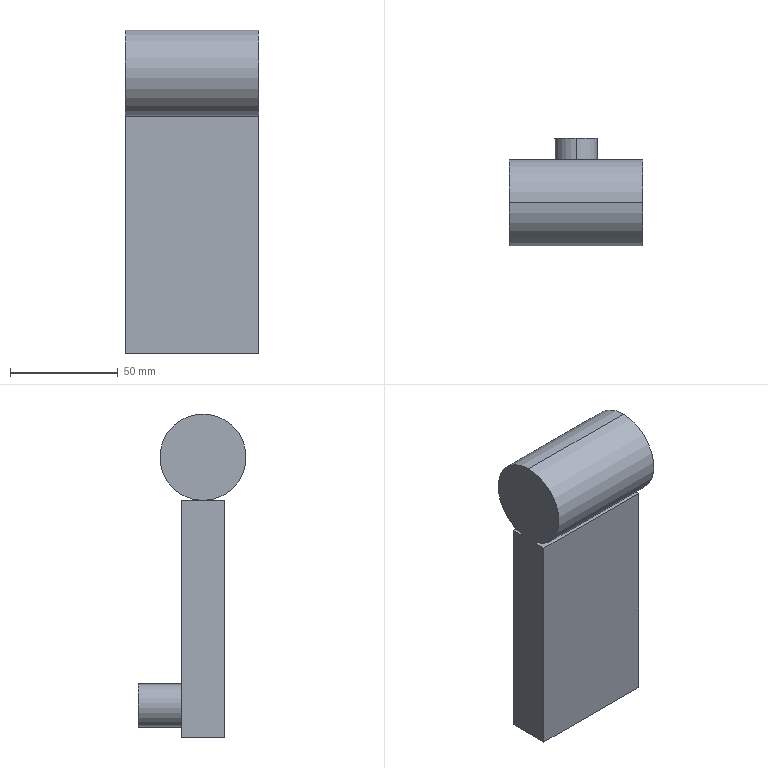Part | SolidWorks | features ICE 2, Extrusion 1 | 2 solids | 13 faces | box 62 x 50 x 150 mm | volume 220595 mm3 | plane 9 | cylinder 4 | commonest cylinder face diameters 20 x2 40 x2
STEP:
#1=CARTESIAN_POINT('',(-31.,0.,150.));
#2=VERTEX_POINT('',#1);
#3=CARTESIAN_POINT('',(-31.,0.,110.));
#4=VERTEX_POINT('',#3);
#5=CARTESIAN_POINT('',(-31.,0.,130.));
#6=DIRECTION('',(-1.,0.,0.));
#7=DIRECTION('',(0.,0.,-1.));
#8=AXIS2_PLACEMENT_3D('',#5,#6,#7);
#9=CIRCLE('',#8,20.);
#10=EDGE_CURVE('',#2,#4,#9,.T.);
#11=ORIENTED_EDGE('',*,*,#10,.F.);
#12=CARTESIAN_POINT('',(31.,0.,150.));
#13=VERTEX_POINT('',#12);
#14=CARTESIAN_POINT('',(-87.569,0.,150.));
#15=DIRECTION('',(1.,0.,0.));
#16=VECTOR('',#15,1000.);
#17=LINE('',#14,#16);
#18=EDGE_CURVE('',#2,#13,#17,.T.);
#19=ORIENTED_EDGE('',*,*,#18,.T.);
#20=CARTESIAN_POINT('',(31.,0.,110.));
#21=VERTEX_POINT('',#20);
#22=CARTESIAN_POINT('',(31.,0.,130.));
#23=DIRECTION('',(1.,0.,0.));
#24=DIRECTION('',(0.,0.,-1.));
#25=AXIS2_PLACEMENT_3D('',#22,#23,#24);
#26=CIRCLE('',#25,20.);
#27=EDGE_CURVE('',#21,#13,#26,.T.);
#28=ORIENTED_EDGE('',*,*,#27,.F.);
#29=CARTESIAN_POINT('',(-87.569,0.,110.));
#30=DIRECTION('',(1.,0.,0.));
#31=VECTOR('',#30,1000.);
#32=LINE('',#29,#31);
#33=EDGE_CURVE('',#4,#21,#32,.T.);
#34=ORIENTED_EDGE('',*,*,#33,.F.);
#35=EDGE_LOOP('',(#11,#19,#28,#34));
#36=FACE_OUTER_BOUND('',#35,.T.);
#37=CARTESIAN_POINT('',(-87.569,0.,130.));
#38=DIRECTION('',(1.,0.,0.));
#39=DIRECTION('',(0.,0.,-1.));
#40=AXIS2_PLACEMENT_3D('',#37,#38,#39);
#41=CYLINDRICAL_SURFACE('',#40,20.);
#42=ADVANCED_FACE('',(#36),#41,.T.);
#43=ORIENTED_EDGE('',*,*,#18,.F.);
#44=CARTESIAN_POINT('',(-31.,0.,130.));
#45=DIRECTION('',(-1.,0.,0.));
#46=DIRECTION('',(0.,0.,-1.));
#47=AXIS2_PLACEMENT_3D('',#44,#45,#46);
#48=CIRCLE('',#47,20.);
#49=EDGE_CURVE('',#4,#2,#48,.T.);
#50=ORIENTED_EDGE('',*,*,#49,.F.);
#51=ORIENTED_EDGE('',*,*,#33,.T.);
#52=CARTESIAN_POINT('',(31.,0.,130.));
#53=DIRECTION('',(1.,0.,0.));
#54=DIRECTION('',(0.,0.,-1.));
#55=AXIS2_PLACEMENT_3D('',#52,#53,#54);
#56=CIRCLE('',#55,20.);
#57=EDGE_CURVE('',#13,#21,#56,.T.);
#58=ORIENTED_EDGE('',*,*,#57,.F.);
#59=EDGE_LOOP('',(#43,#50,#51,#58));
#60=FACE_OUTER_BOUND('',#59,.T.);
#61=CARTESIAN_POINT('',(-87.569,0.,130.));
#62=DIRECTION('',(1.,0.,0.));
#63=DIRECTION('',(0.,0.,-1.));
#64=AXIS2_PLACEMENT_3D('',#61,#62,#63);
#65=CYLINDRICAL_SURFACE('',#64,20.);
#66=ADVANCED_FACE('',(#60),#65,.T.);
#67=ORIENTED_EDGE('',*,*,#27,.T.);
#68=ORIENTED_EDGE('',*,*,#57,.T.);
#69=EDGE_LOOP('',(#67,#68));
#70=FACE_OUTER_BOUND('',#69,.T.);
#71=CARTESIAN_POINT('',(31.,0.,130.));
#72=DIRECTION('',(1.,0.,0.));
#73=DIRECTION('',(0.,0.,-1.));
#74=AXIS2_PLACEMENT_3D('',#71,#72,#73);
#75=PLANE('',#74);
#76=ADVANCED_FACE('',(#70),#75,.T.);
#77=ORIENTED_EDGE('',*,*,#49,.T.);
#78=ORIENTED_EDGE('',*,*,#10,.T.);
#79=EDGE_LOOP('',(#77,#78));
#80=FACE_OUTER_BOUND('',#79,.T.);
#81=CARTESIAN_POINT('',(-31.,-10.,110.));
#82=DIRECTION('',(1.,0.,0.));
#83=DIRECTION('',(0.,0.,-1.));
#84=AXIS2_PLACEMENT_3D('',#81,#82,#83);
#85=PLANE('',#84);
#86=ADVANCED_FACE('',(#80),#85,.F.);
#87=CLOSED_SHELL('',(#42,#66,#76,#86));
#88=MANIFOLD_SOLID_BREP('',#87);
#89=CARTESIAN_POINT('',(0.,30.,25.));
#90=VERTEX_POINT('',#89);
#91=CARTESIAN_POINT('',(0.,30.,5.));
#92=VERTEX_POINT('',#91);
#93=CARTESIAN_POINT('',(0.,30.,15.));
#94=DIRECTION('',(0.,1.,0.));
#95=DIRECTION('',(0.,0.,1.));
#96=AXIS2_PLACEMENT_3D('',#93,#94,#95);
#97=CIRCLE('',#96,10.);
#98=EDGE_CURVE('',#90,#92,#97,.T.);
#99=ORIENTED_EDGE('',*,*,#98,.F.);
#100=CARTESIAN_POINT('',(0.,10.,25.));
#101=VERTEX_POINT('',#100);
#102=CARTESIAN_POINT('',(0.,30.,25.));
#103=DIRECTION('',(0.,-1.,0.));
#104=VECTOR('',#103,1000.);
#105=LINE('',#102,#104);
#106=EDGE_CURVE('',#90,#101,#105,.T.);
#107=ORIENTED_EDGE('',*,*,#106,.T.);
#108=CARTESIAN_POINT('',(0.,10.,5.));
#109=VERTEX_POINT('',#108);
#110=CARTESIAN_POINT('',(0.,10.,15.));
#111=DIRECTION('',(0.,1.,0.));
#112=DIRECTION('',(0.,0.,-1.));
#113=AXIS2_PLACEMENT_3D('',#110,#111,#112);
#114=CIRCLE('',#113,10.);
#115=EDGE_CURVE('',#101,#109,#114,.T.);
#116=ORIENTED_EDGE('',*,*,#115,.T.);
#117=CARTESIAN_POINT('',(0.,30.,5.));
#118=DIRECTION('',(0.,-1.,0.));
#119=VECTOR('',#118,1000.);
#120=LINE('',#117,#119);
#121=EDGE_CURVE('',#92,#109,#120,.T.);
#122=ORIENTED_EDGE('',*,*,#121,.F.);
#123=EDGE_LOOP('',(#99,#107,#116,#122));
#124=FACE_OUTER_BOUND('',#123,.T.);
#125=CARTESIAN_POINT('',(0.,30.,15.));
#126=DIRECTION('',(0.,-1.,0.));
#127=DIRECTION('',(0.,0.,-1.));
#128=AXIS2_PLACEMENT_3D('',#125,#126,#127);
#129=CYLINDRICAL_SURFACE('',#128,10.);
#130=ADVANCED_FACE('',(#124),#129,.T.);
#131=CARTESIAN_POINT('',(31.,-10.,0.));
#132=VERTEX_POINT('',#131);
#133=CARTESIAN_POINT('',(31.,10.,0.));
#134=VERTEX_POINT('',#133);
#135=CARTESIAN_POINT('',(31.,-10.,0.));
#136=DIRECTION('',(0.,1.,0.));
#137=VECTOR('',#136,1000.);
#138=LINE('',#135,#137);
#139=EDGE_CURVE('',#132,#134,#138,.T.);
#140=ORIENTED_EDGE('',*,*,#139,.T.);
#141=CARTESIAN_POINT('',(31.,10.,110.));
#142=VERTEX_POINT('',#141);
#143=CARTESIAN_POINT('',(31.,10.,110.));
#144=DIRECTION('',(0.,0.,-1.));
#145=VECTOR('',#144,1000.);
#146=LINE('',#143,#145);
#147=EDGE_CURVE('',#142,#134,#146,.T.);
#148=ORIENTED_EDGE('',*,*,#147,.F.);
#149=CARTESIAN_POINT('',(31.,-10.,110.));
#150=VERTEX_POINT('',#149);
#151=CARTESIAN_POINT('',(31.,-10.,110.));
#152=DIRECTION('',(0.,1.,0.));
#153=VECTOR('',#152,1000.);
#154=LINE('',#151,#153);
#155=EDGE_CURVE('',#150,#142,#154,.T.);
#156=ORIENTED_EDGE('',*,*,#155,.F.);
#157=CARTESIAN_POINT('',(31.,-10.,110.));
#158=DIRECTION('',(0.,0.,-1.));
#159=VECTOR('',#158,1000.);
#160=LINE('',#157,#159);
#161=EDGE_CURVE('',#150,#132,#160,.T.);
#162=ORIENTED_EDGE('',*,*,#161,.T.);
#163=EDGE_LOOP('',(#140,#148,#156,#162));
#164=FACE_OUTER_BOUND('',#163,.T.);
#165=CARTESIAN_POINT('',(31.,-10.,110.));
#166=DIRECTION('',(-1.,0.,0.));
#167=DIRECTION('',(0.,0.,1.));
#168=AXIS2_PLACEMENT_3D('',#165,#166,#167);
#169=PLANE('',#168);
#170=ADVANCED_FACE('',(#164),#169,.F.);
#171=CARTESIAN_POINT('',(0.,10.,15.));
#172=DIRECTION('',(0.,1.,0.));
#173=DIRECTION('',(0.,0.,-1.));
#174=AXIS2_PLACEMENT_3D('',#171,#172,#173);
#175=CIRCLE('',#174,10.);
#176=EDGE_CURVE('',#109,#101,#175,.T.);
#177=ORIENTED_EDGE('',*,*,#176,.F.);
#178=ORIENTED_EDGE('',*,*,#115,.F.);
#179=EDGE_LOOP('',(#177,#178));
#180=FACE_BOUND('',#179,.T.);
#181=CARTESIAN_POINT('',(-31.,10.,0.));
#182=VERTEX_POINT('',#181);
#183=CARTESIAN_POINT('',(-31.,10.,0.));
#184=DIRECTION('',(-1.,0.,0.));
#185=VECTOR('',#184,1000.);
#186=LINE('',#183,#185);
#187=EDGE_CURVE('',#134,#182,#186,.T.);
#188=ORIENTED_EDGE('',*,*,#187,.T.);
#189=CARTESIAN_POINT('',(-31.,10.,110.));
#190=VERTEX_POINT('',#189);
#191=CARTESIAN_POINT('',(-31.,10.,110.));
#192=DIRECTION('',(0.,0.,-1.));
#193=VECTOR('',#192,1000.);
#194=LINE('',#191,#193);
#195=EDGE_CURVE('',#190,#182,#194,.T.);
#196=ORIENTED_EDGE('',*,*,#195,.F.);
#197=CARTESIAN_POINT('',(-31.,10.,110.));
#198=DIRECTION('',(-1.,0.,0.));
#199=VECTOR('',#198,1000.);
#200=LINE('',#197,#199);
#201=EDGE_CURVE('',#142,#190,#200,.T.);
#202=ORIENTED_EDGE('',*,*,#201,.F.);
#203=ORIENTED_EDGE('',*,*,#147,.T.);
#204=EDGE_LOOP('',(#188,#196,#202,#203));
#205=FACE_OUTER_BOUND('',#204,.T.);
#206=CARTESIAN_POINT('',(-31.,10.,110.));
#207=DIRECTION('',(0.,-1.,0.));
#208=DIRECTION('',(0.,0.,-1.));
#209=AXIS2_PLACEMENT_3D('',#206,#207,#208);
#210=PLANE('',#209);
#211=ADVANCED_FACE('',(#180,#205),#210,.F.);
#212=CARTESIAN_POINT('',(-31.,-10.,0.));
#213=VERTEX_POINT('',#212);
#214=CARTESIAN_POINT('',(-31.,-10.,0.));
#215=DIRECTION('',(0.,-1.,0.));
#216=VECTOR('',#215,1000.);
#217=LINE('',#214,#216);
#218=EDGE_CURVE('',#182,#213,#217,.T.);
#219=ORIENTED_EDGE('',*,*,#218,.T.);
#220=CARTESIAN_POINT('',(-31.,-10.,110.));
#221=VERTEX_POINT('',#220);
#222=CARTESIAN_POINT('',(-31.,-10.,110.));
#223=DIRECTION('',(0.,0.,-1.));
#224=VECTOR('',#223,1000.);
#225=LINE('',#222,#224);
#226=EDGE_CURVE('',#221,#213,#225,.T.);
#227=ORIENTED_EDGE('',*,*,#226,.F.);
#228=CARTESIAN_POINT('',(-31.,-10.,110.));
#229=DIRECTION('',(0.,-1.,0.));
#230=VECTOR('',#229,1000.);
#231=LINE('',#228,#230);
#232=EDGE_CURVE('',#190,#221,#231,.T.);
#233=ORIENTED_EDGE('',*,*,#232,.F.);
#234=ORIENTED_EDGE('',*,*,#195,.T.);
#235=EDGE_LOOP('',(#219,#227,#233,#234));
#236=FACE_OUTER_BOUND('',#235,.T.);
#237=CARTESIAN_POINT('',(-31.,-10.,110.));
#238=DIRECTION('',(1.,0.,0.));
#239=DIRECTION('',(0.,0.,-1.));
#240=AXIS2_PLACEMENT_3D('',#237,#238,#239);
#241=PLANE('',#240);
#242=ADVANCED_FACE('',(#236),#241,.F.);
#243=CARTESIAN_POINT('',(-31.,-10.,0.));
#244=DIRECTION('',(1.,0.,0.));
#245=VECTOR('',#244,1000.);
#246=LINE('',#243,#245);
#247=EDGE_CURVE('',#213,#132,#246,.T.);
#248=ORIENTED_EDGE('',*,*,#247,.T.);
#249=ORIENTED_EDGE('',*,*,#161,.F.);
#250=CARTESIAN_POINT('',(-31.,-10.,110.));
#251=DIRECTION('',(1.,0.,0.));
#252=VECTOR('',#251,1000.);
#253=LINE('',#250,#252);
#254=EDGE_CURVE('',#221,#150,#253,.T.);
#255=ORIENTED_EDGE('',*,*,#254,.F.);
#256=ORIENTED_EDGE('',*,*,#226,.T.);
#257=EDGE_LOOP('',(#248,#249,#255,#256));
#258=FACE_OUTER_BOUND('',#257,.T.);
#259=CARTESIAN_POINT('',(-31.,-10.,110.));
#260=DIRECTION('',(0.,1.,0.));
#261=DIRECTION('',(0.,0.,1.));
#262=AXIS2_PLACEMENT_3D('',#259,#260,#261);
#263=PLANE('',#262);
#264=ADVANCED_FACE('',(#258),#263,.F.);
#265=ORIENTED_EDGE('',*,*,#155,.T.);
#266=ORIENTED_EDGE('',*,*,#201,.T.);
#267=ORIENTED_EDGE('',*,*,#232,.T.);
#268=ORIENTED_EDGE('',*,*,#254,.T.);
#269=EDGE_LOOP('',(#265,#266,#267,#268));
#270=FACE_OUTER_BOUND('',#269,.T.);
#271=CARTESIAN_POINT('',(0.,0.,110.));
#272=DIRECTION('',(0.,0.,-1.));
#273=DIRECTION('',(-1.,0.,0.));
#274=AXIS2_PLACEMENT_3D('',#271,#272,#273);
#275=PLANE('',#274);
#276=ADVANCED_FACE('',(#270),#275,.F.);
#277=ORIENTED_EDGE('',*,*,#139,.F.);
#278=ORIENTED_EDGE('',*,*,#247,.F.);
#279=ORIENTED_EDGE('',*,*,#218,.F.);
#280=ORIENTED_EDGE('',*,*,#187,.F.);
#281=EDGE_LOOP('',(#277,#278,#279,#280));
#282=FACE_OUTER_BOUND('',#281,.T.);
#283=CARTESIAN_POINT('',(0.,0.,0.));
#284=DIRECTION('',(0.,0.,-1.));
#285=DIRECTION('',(-1.,0.,0.));
#286=AXIS2_PLACEMENT_3D('',#283,#284,#285);
#287=PLANE('',#286);
#288=ADVANCED_FACE('',(#282),#287,.T.);
#289=ORIENTED_EDGE('',*,*,#106,.F.);
#290=CARTESIAN_POINT('',(0.,30.,15.));
#291=DIRECTION('',(0.,1.,0.));
#292=DIRECTION('',(0.,0.,1.));
#293=AXIS2_PLACEMENT_3D('',#290,#291,#292);
#294=CIRCLE('',#293,10.);
#295=EDGE_CURVE('',#92,#90,#294,.T.);
#296=ORIENTED_EDGE('',*,*,#295,.F.);
#297=ORIENTED_EDGE('',*,*,#121,.T.);
#298=ORIENTED_EDGE('',*,*,#176,.T.);
#299=EDGE_LOOP('',(#289,#296,#297,#298));
#300=FACE_OUTER_BOUND('',#299,.T.);
#301=CARTESIAN_POINT('',(0.,30.,15.));
#302=DIRECTION('',(0.,-1.,0.));
#303=DIRECTION('',(0.,0.,-1.));
#304=AXIS2_PLACEMENT_3D('',#301,#302,#303);
#305=CYLINDRICAL_SURFACE('',#304,10.);
#306=ADVANCED_FACE('',(#300),#305,.T.);
#307=ORIENTED_EDGE('',*,*,#295,.T.);
#308=ORIENTED_EDGE('',*,*,#98,.T.);
#309=EDGE_LOOP('',(#307,#308));
#310=FACE_OUTER_BOUND('',#309,.T.);
#311=CARTESIAN_POINT('',(0.,30.,15.));
#312=DIRECTION('',(0.,1.,0.));
#313=DIRECTION('',(0.,0.,1.));
#314=AXIS2_PLACEMENT_3D('',#311,#312,#313);
#315=PLANE('',#314);
#316=ADVANCED_FACE('',(#310),#315,.T.);
#317=CLOSED_SHELL('',(#130,#170,#211,#242,#264,#276,#288,#306,#316));
#318=MANIFOLD_SOLID_BREP('',#317);
#319=CARTESIAN_POINT('',(0.,0.,0.));
#320=DIRECTION('',(0.,0.,1.));
#321=DIRECTION('',(1.,0.,0.));
#322=AXIS2_PLACEMENT_3D('',#319,#320,#321);
#323=(LENGTH_UNIT()NAMED_UNIT(*)SI_UNIT(.MILLI.,.METRE.));
#324=UNCERTAINTY_MEASURE_WITH_UNIT(LENGTH_MEASURE(0.00001),#323,'','');
#325=(NAMED_UNIT(*)PLANE_ANGLE_UNIT()SI_UNIT($,.RADIAN.));
#326=(NAMED_UNIT(*)SI_UNIT($,.STERADIAN.)SOLID_ANGLE_UNIT());
#327=(GEOMETRIC_REPRESENTATION_CONTEXT(3)GLOBAL_UNCERTAINTY_ASSIGNED_CONTEXT((#324))GLOBAL_UNIT_ASSIGNED_CONTEXT((#323,#325,#326))REPRESENTATION_CONTEXT('',''));
#328=ADVANCED_BREP_SHAPE_REPRESENTATION('',(#88,#318,#322),#327);